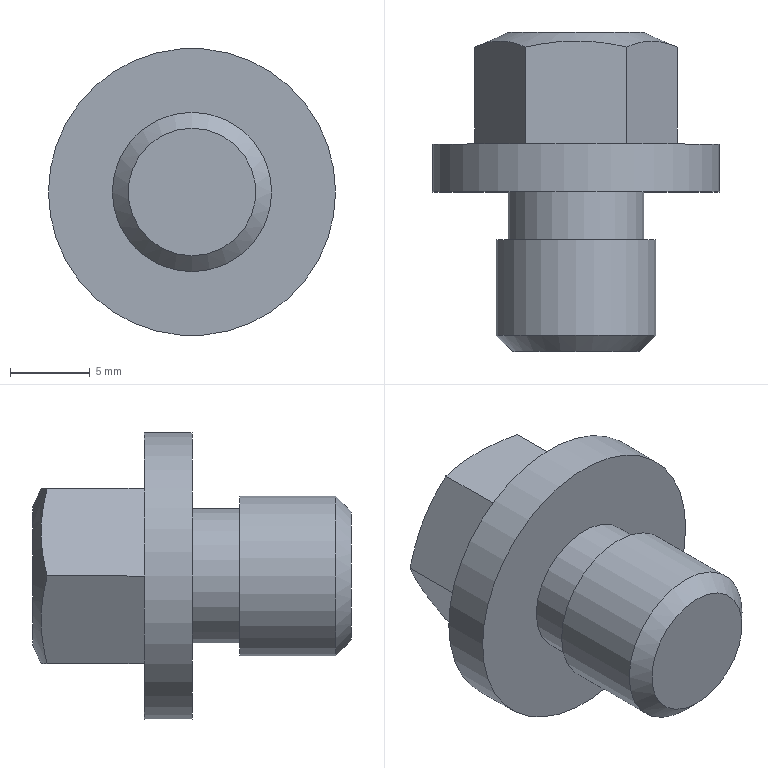Part | NX | features DATUM_CSYS 6, SKETCH 5, EXTRUDE 4, CHAMFER 1, SWP104 1 | 1 solid | 16 faces | box 18 x 20 x 18 mm | volume 2187 mm3 | plane 11 | cylinder 3 | cone 2 | commonest cylinder face diameters 8.5 x1 10 x1 18 x1
STEP:
#1=CARTESIAN_POINT('',(0.,-6.,-5.));
#2=VERTEX_POINT('',#1);
#3=CARTESIAN_POINT('',(0.,-6.,0.));
#4=DIRECTION('',(0.,-1.,0.));
#5=DIRECTION('',(0.,0.,-1.));
#6=AXIS2_PLACEMENT_3D('',#3,#4,#5);
#7=CIRCLE('',#6,5.);
#8=EDGE_CURVE('',#2,#2,#7,.F.);
#9=ORIENTED_EDGE('',*,*,#8,.T.);
#10=EDGE_LOOP('',(#9));
#11=FACE_BOUND('',#10,.T.);
#12=CARTESIAN_POINT('',(5.,0.,0.));
#13=VERTEX_POINT('',#12);
#14=CARTESIAN_POINT('',(0.,0.,0.));
#15=DIRECTION('',(0.,-1.,0.));
#16=DIRECTION('',(1.,0.,0.));
#17=AXIS2_PLACEMENT_3D('',#14,#15,#16);
#18=CIRCLE('',#17,5.);
#19=EDGE_CURVE('',#13,#13,#18,.T.);
#20=ORIENTED_EDGE('',*,*,#19,.T.);
#21=EDGE_LOOP('',(#20));
#22=FACE_BOUND('',#21,.T.);
#23=CARTESIAN_POINT('',(0.,-7.,0.));
#24=DIRECTION('',(0.,1.,0.));
#25=DIRECTION('',(0.,0.,1.));
#26=AXIS2_PLACEMENT_3D('',#23,#24,#25);
#27=CYLINDRICAL_SURFACE('',#26,5.);
#28=ADVANCED_FACE('',(#11,#22),#27,.T.);
#29=CARTESIAN_POINT('',(0.,-7.,-4.));
#30=VERTEX_POINT('',#29);
#31=CARTESIAN_POINT('',(0.,-7.,0.));
#32=DIRECTION('',(0.,-1.,0.));
#33=DIRECTION('',(0.,0.,-1.));
#34=AXIS2_PLACEMENT_3D('',#31,#32,#33);
#35=CIRCLE('',#34,4.);
#36=EDGE_CURVE('',#30,#30,#35,.T.);
#37=ORIENTED_EDGE('',*,*,#36,.T.);
#38=EDGE_LOOP('',(#37));
#39=FACE_BOUND('',#38,.T.);
#40=CARTESIAN_POINT('',(0.,-7.,0.));
#41=DIRECTION('',(0.,-1.,0.));
#42=DIRECTION('',(0.,0.,-1.));
#43=AXIS2_PLACEMENT_3D('',#40,#41,#42);
#44=PLANE('',#43);
#45=ADVANCED_FACE('',(#39),#44,.T.);
#46=CARTESIAN_POINT('',(4.25,0.,0.));
#47=VERTEX_POINT('',#46);
#48=CARTESIAN_POINT('',(0.,0.,0.));
#49=DIRECTION('',(0.,1.,0.));
#50=DIRECTION('',(1.,0.,0.));
#51=AXIS2_PLACEMENT_3D('',#48,#49,#50);
#52=CIRCLE('',#51,4.25);
#53=EDGE_CURVE('',#47,#47,#52,.T.);
#54=ORIENTED_EDGE('',*,*,#53,.F.);
#55=EDGE_LOOP('',(#54));
#56=FACE_BOUND('',#55,.T.);
#57=ORIENTED_EDGE('',*,*,#19,.F.);
#58=EDGE_LOOP('',(#57));
#59=FACE_BOUND('',#58,.T.);
#60=CARTESIAN_POINT('',(0.,0.,0.));
#61=DIRECTION('',(0.,-1.,0.));
#62=DIRECTION('',(0.,0.,-1.));
#63=AXIS2_PLACEMENT_3D('',#60,#61,#62);
#64=PLANE('',#63);
#65=ADVANCED_FACE('',(#56,#59),#64,.F.);
#66=CARTESIAN_POINT('',(4.25,3.,0.));
#67=VERTEX_POINT('',#66);
#68=CARTESIAN_POINT('',(0.,3.,0.));
#69=DIRECTION('',(0.,1.,0.));
#70=DIRECTION('',(1.,0.,0.));
#71=AXIS2_PLACEMENT_3D('',#68,#69,#70);
#72=CIRCLE('',#71,4.25);
#73=EDGE_CURVE('',#67,#67,#72,.T.);
#74=ORIENTED_EDGE('',*,*,#73,.F.);
#75=EDGE_LOOP('',(#74));
#76=FACE_BOUND('',#75,.T.);
#77=ORIENTED_EDGE('',*,*,#53,.T.);
#78=EDGE_LOOP('',(#77));
#79=FACE_BOUND('',#78,.T.);
#80=CARTESIAN_POINT('',(0.,3.,0.));
#81=DIRECTION('',(0.,-1.,0.));
#82=DIRECTION('',(0.,0.,-1.));
#83=AXIS2_PLACEMENT_3D('',#80,#81,#82);
#84=CYLINDRICAL_SURFACE('',#83,4.25);
#85=ADVANCED_FACE('',(#76,#79),#84,.T.);
#86=CARTESIAN_POINT('',(9.,6.,0.));
#87=VERTEX_POINT('',#86);
#88=CARTESIAN_POINT('',(0.,6.,0.));
#89=DIRECTION('',(0.,1.,0.));
#90=DIRECTION('',(1.,0.,0.));
#91=AXIS2_PLACEMENT_3D('',#88,#89,#90);
#92=CIRCLE('',#91,9.);
#93=EDGE_CURVE('',#87,#87,#92,.T.);
#94=ORIENTED_EDGE('',*,*,#93,.F.);
#95=EDGE_LOOP('',(#94));
#96=FACE_BOUND('',#95,.T.);
#97=CARTESIAN_POINT('',(9.,3.,0.));
#98=VERTEX_POINT('',#97);
#99=CARTESIAN_POINT('',(0.,3.,0.));
#100=DIRECTION('',(0.,1.,0.));
#101=DIRECTION('',(1.,0.,0.));
#102=AXIS2_PLACEMENT_3D('',#99,#100,#101);
#103=CIRCLE('',#102,9.);
#104=EDGE_CURVE('',#98,#98,#103,.T.);
#105=ORIENTED_EDGE('',*,*,#104,.T.);
#106=EDGE_LOOP('',(#105));
#107=FACE_BOUND('',#106,.T.);
#108=CARTESIAN_POINT('',(0.,6.,0.));
#109=DIRECTION('',(0.,-1.,0.));
#110=DIRECTION('',(0.,0.,-1.));
#111=AXIS2_PLACEMENT_3D('',#108,#109,#110);
#112=CYLINDRICAL_SURFACE('',#111,9.);
#113=ADVANCED_FACE('',(#96,#107),#112,.T.);
#114=CARTESIAN_POINT('',(-3.18,6.,-5.508));
#115=VERTEX_POINT('',#114);
#116=CARTESIAN_POINT('',(-6.36,6.,0.));
#117=VERTEX_POINT('',#116);
#118=CARTESIAN_POINT('',(-3.18,6.,-5.508));
#119=DIRECTION('',(-0.5,0.,0.866));
#120=VECTOR('',#119,1000.);
#121=LINE('',#118,#120);
#122=EDGE_CURVE('',#115,#117,#121,.T.);
#123=ORIENTED_EDGE('',*,*,#122,.F.);
#124=CARTESIAN_POINT('',(3.18,6.,-5.508));
#125=VERTEX_POINT('',#124);
#126=CARTESIAN_POINT('',(3.18,6.,-5.508));
#127=DIRECTION('',(-1.,0.,0.));
#128=VECTOR('',#127,1000.);
#129=LINE('',#126,#128);
#130=EDGE_CURVE('',#125,#115,#129,.T.);
#131=ORIENTED_EDGE('',*,*,#130,.F.);
#132=CARTESIAN_POINT('',(6.36,6.,0.));
#133=VERTEX_POINT('',#132);
#134=CARTESIAN_POINT('',(6.36,6.,0.));
#135=DIRECTION('',(-0.5,0.,-0.866));
#136=VECTOR('',#135,1000.);
#137=LINE('',#134,#136);
#138=EDGE_CURVE('',#133,#125,#137,.T.);
#139=ORIENTED_EDGE('',*,*,#138,.F.);
#140=CARTESIAN_POINT('',(3.18,6.,5.508));
#141=VERTEX_POINT('',#140);
#142=CARTESIAN_POINT('',(3.18,6.,5.508));
#143=DIRECTION('',(0.5,0.,-0.866));
#144=VECTOR('',#143,1000.);
#145=LINE('',#142,#144);
#146=EDGE_CURVE('',#141,#133,#145,.T.);
#147=ORIENTED_EDGE('',*,*,#146,.F.);
#148=CARTESIAN_POINT('',(-3.18,6.,5.508));
#149=VERTEX_POINT('',#148);
#150=CARTESIAN_POINT('',(-3.18,6.,5.508));
#151=DIRECTION('',(1.,0.,0.));
#152=VECTOR('',#151,1000.);
#153=LINE('',#150,#152);
#154=EDGE_CURVE('',#149,#141,#153,.T.);
#155=ORIENTED_EDGE('',*,*,#154,.F.);
#156=CARTESIAN_POINT('',(-6.36,6.,0.));
#157=DIRECTION('',(0.5,0.,0.866));
#158=VECTOR('',#157,1000.);
#159=LINE('',#156,#158);
#160=EDGE_CURVE('',#117,#149,#159,.T.);
#161=ORIENTED_EDGE('',*,*,#160,.F.);
#162=EDGE_LOOP('',(#123,#131,#139,#147,#155,#161));
#163=FACE_BOUND('',#162,.T.);
#164=ORIENTED_EDGE('',*,*,#93,.T.);
#165=EDGE_LOOP('',(#164));
#166=FACE_BOUND('',#165,.T.);
#167=CARTESIAN_POINT('',(0.,6.,0.));
#168=DIRECTION('',(0.,1.,0.));
#169=DIRECTION('',(0.,0.,1.));
#170=AXIS2_PLACEMENT_3D('',#167,#168,#169);
#171=PLANE('',#170);
#172=ADVANCED_FACE('',(#163,#166),#171,.T.);
#173=ORIENTED_EDGE('',*,*,#73,.T.);
#174=EDGE_LOOP('',(#173));
#175=FACE_BOUND('',#174,.T.);
#176=ORIENTED_EDGE('',*,*,#104,.F.);
#177=EDGE_LOOP('',(#176));
#178=FACE_BOUND('',#177,.T.);
#179=CARTESIAN_POINT('',(0.,3.,0.));
#180=DIRECTION('',(0.,1.,0.));
#181=DIRECTION('',(0.,0.,1.));
#182=AXIS2_PLACEMENT_3D('',#179,#180,#181);
#183=PLANE('',#182);
#184=ADVANCED_FACE('',(#175,#178),#183,.F.);
#185=CARTESIAN_POINT('',(-6.36,12.082,0.));
#186=VERTEX_POINT('',#185);
#187=CARTESIAN_POINT('',(-6.36,13.,0.));
#188=DIRECTION('',(0.,-1.,0.));
#189=VECTOR('',#188,1000.);
#190=LINE('',#187,#189);
#191=EDGE_CURVE('',#186,#117,#190,.T.);
#192=ORIENTED_EDGE('',*,*,#191,.F.);
#193=CARTESIAN_POINT('',(-3.18,12.082,-5.508));
#194=VERTEX_POINT('',#193);
#195=CARTESIAN_POINT('',(-6.36,12.082,0.));
#196=CARTESIAN_POINT('',(-5.835,12.314,-0.9096));
#197=CARTESIAN_POINT('',(-4.781,12.602,-2.734));
#198=CARTESIAN_POINT('',(-3.707,12.315,-4.595));
#199=CARTESIAN_POINT('',(-3.18,12.082,-5.508));
#200=B_SPLINE_CURVE_WITH_KNOTS('',3,(#195,#196,#197,#198,#199),.UNSPECIFIED.,.F.,.F.,(4,1,4),(0.000000233,0.003183,0.006366),.UNSPECIFIED.);
#201=EDGE_CURVE('',#186,#194,#200,.T.);
#202=ORIENTED_EDGE('',*,*,#201,.T.);
#203=CARTESIAN_POINT('',(-3.18,13.,-5.508));
#204=DIRECTION('',(0.,-1.,0.));
#205=VECTOR('',#204,1000.);
#206=LINE('',#203,#205);
#207=EDGE_CURVE('',#194,#115,#206,.T.);
#208=ORIENTED_EDGE('',*,*,#207,.T.);
#209=ORIENTED_EDGE('',*,*,#122,.T.);
#210=EDGE_LOOP('',(#192,#202,#208,#209));
#211=FACE_BOUND('',#210,.T.);
#212=CARTESIAN_POINT('',(-3.18,13.,-5.508));
#213=DIRECTION('',(0.866,0.,0.5));
#214=DIRECTION('',(0.5,0.,-0.866));
#215=AXIS2_PLACEMENT_3D('',#212,#213,#214);
#216=PLANE('',#215);
#217=ADVANCED_FACE('',(#211),#216,.F.);
#218=CARTESIAN_POINT('',(-3.18,12.082,5.508));
#219=VERTEX_POINT('',#218);
#220=CARTESIAN_POINT('',(-3.18,13.,5.508));
#221=DIRECTION('',(0.,-1.,0.));
#222=VECTOR('',#221,1000.);
#223=LINE('',#220,#222);
#224=EDGE_CURVE('',#219,#149,#223,.T.);
#225=ORIENTED_EDGE('',*,*,#224,.F.);
#226=CARTESIAN_POINT('',(-3.18,12.082,5.508));
#227=CARTESIAN_POINT('',(-3.705,12.314,4.598));
#228=CARTESIAN_POINT('',(-4.759,12.602,2.774));
#229=CARTESIAN_POINT('',(-5.833,12.315,0.9126));
#230=CARTESIAN_POINT('',(-6.36,12.082,0.));
#231=B_SPLINE_CURVE_WITH_KNOTS('',3,(#226,#227,#228,#229,#230),.UNSPECIFIED.,.F.,.F.,(4,1,4),(0.000000233,0.003183,0.006366),.UNSPECIFIED.);
#232=EDGE_CURVE('',#219,#186,#231,.T.);
#233=ORIENTED_EDGE('',*,*,#232,.T.);
#234=ORIENTED_EDGE('',*,*,#191,.T.);
#235=ORIENTED_EDGE('',*,*,#160,.T.);
#236=EDGE_LOOP('',(#225,#233,#234,#235));
#237=FACE_BOUND('',#236,.T.);
#238=CARTESIAN_POINT('',(-6.36,13.,0.));
#239=DIRECTION('',(0.866,0.,-0.5));
#240=DIRECTION('',(-0.5,0.,-0.866));
#241=AXIS2_PLACEMENT_3D('',#238,#239,#240);
#242=PLANE('',#241);
#243=ADVANCED_FACE('',(#237),#242,.F.);
#244=CARTESIAN_POINT('',(3.18,12.082,5.508));
#245=VERTEX_POINT('',#244);
#246=CARTESIAN_POINT('',(3.18,13.,5.508));
#247=DIRECTION('',(0.,-1.,0.));
#248=VECTOR('',#247,1000.);
#249=LINE('',#246,#248);
#250=EDGE_CURVE('',#245,#141,#249,.T.);
#251=ORIENTED_EDGE('',*,*,#250,.F.);
#252=CARTESIAN_POINT('',(-3.18,12.082,5.508));
#253=CARTESIAN_POINT('',(-2.133,12.313,5.508));
#254=CARTESIAN_POINT('',(-0.001857,12.604,5.508));
#255=CARTESIAN_POINT('',(2.136,12.313,5.508));
#256=CARTESIAN_POINT('',(3.18,12.082,5.508));
#257=B_SPLINE_CURVE_WITH_KNOTS('',3,(#252,#253,#254,#255,#256),.UNSPECIFIED.,.F.,.F.,(4,1,4),(0.005432,0.008641,0.01185),.UNSPECIFIED.);
#258=EDGE_CURVE('',#245,#219,#257,.F.);
#259=ORIENTED_EDGE('',*,*,#258,.T.);
#260=ORIENTED_EDGE('',*,*,#224,.T.);
#261=ORIENTED_EDGE('',*,*,#154,.T.);
#262=EDGE_LOOP('',(#251,#259,#260,#261));
#263=FACE_BOUND('',#262,.T.);
#264=CARTESIAN_POINT('',(-3.18,13.,5.508));
#265=DIRECTION('',(0.,0.,-1.));
#266=DIRECTION('',(-1.,0.,0.));
#267=AXIS2_PLACEMENT_3D('',#264,#265,#266);
#268=PLANE('',#267);
#269=ADVANCED_FACE('',(#263),#268,.F.);
#270=CARTESIAN_POINT('',(6.36,12.082,0.));
#271=VERTEX_POINT('',#270);
#272=CARTESIAN_POINT('',(6.36,13.,0.));
#273=DIRECTION('',(0.,-1.,0.));
#274=VECTOR('',#273,1000.);
#275=LINE('',#272,#274);
#276=EDGE_CURVE('',#271,#133,#275,.T.);
#277=ORIENTED_EDGE('',*,*,#276,.F.);
#278=CARTESIAN_POINT('',(6.36,12.082,0.));
#279=CARTESIAN_POINT('',(5.835,12.314,0.9096));
#280=CARTESIAN_POINT('',(4.781,12.602,2.734));
#281=CARTESIAN_POINT('',(3.707,12.315,4.595));
#282=CARTESIAN_POINT('',(3.18,12.082,5.508));
#283=B_SPLINE_CURVE_WITH_KNOTS('',3,(#278,#279,#280,#281,#282),.UNSPECIFIED.,.F.,.F.,(4,1,4),(0.000000233,0.003183,0.006366),.UNSPECIFIED.);
#284=EDGE_CURVE('',#271,#245,#283,.T.);
#285=ORIENTED_EDGE('',*,*,#284,.T.);
#286=ORIENTED_EDGE('',*,*,#250,.T.);
#287=ORIENTED_EDGE('',*,*,#146,.T.);
#288=EDGE_LOOP('',(#277,#285,#286,#287));
#289=FACE_BOUND('',#288,.T.);
#290=CARTESIAN_POINT('',(3.18,13.,5.508));
#291=DIRECTION('',(-0.866,0.,-0.5));
#292=DIRECTION('',(-0.5,0.,0.866));
#293=AXIS2_PLACEMENT_3D('',#290,#291,#292);
#294=PLANE('',#293);
#295=ADVANCED_FACE('',(#289),#294,.F.);
#296=CARTESIAN_POINT('',(3.18,12.082,-5.508));
#297=VERTEX_POINT('',#296);
#298=CARTESIAN_POINT('',(3.18,13.,-5.508));
#299=DIRECTION('',(0.,-1.,0.));
#300=VECTOR('',#299,1000.);
#301=LINE('',#298,#300);
#302=EDGE_CURVE('',#297,#125,#301,.T.);
#303=ORIENTED_EDGE('',*,*,#302,.F.);
#304=CARTESIAN_POINT('',(3.18,12.082,-5.508));
#305=CARTESIAN_POINT('',(3.705,12.314,-4.598));
#306=CARTESIAN_POINT('',(4.759,12.602,-2.774));
#307=CARTESIAN_POINT('',(5.833,12.315,-0.9126));
#308=CARTESIAN_POINT('',(6.36,12.082,0.));
#309=B_SPLINE_CURVE_WITH_KNOTS('',3,(#304,#305,#306,#307,#308),.UNSPECIFIED.,.F.,.F.,(4,1,4),(0.000000233,0.003183,0.006366),.UNSPECIFIED.);
#310=EDGE_CURVE('',#297,#271,#309,.T.);
#311=ORIENTED_EDGE('',*,*,#310,.T.);
#312=ORIENTED_EDGE('',*,*,#276,.T.);
#313=ORIENTED_EDGE('',*,*,#138,.T.);
#314=EDGE_LOOP('',(#303,#311,#312,#313));
#315=FACE_BOUND('',#314,.T.);
#316=CARTESIAN_POINT('',(6.36,13.,0.));
#317=DIRECTION('',(-0.866,0.,0.5));
#318=DIRECTION('',(0.5,0.,0.866));
#319=AXIS2_PLACEMENT_3D('',#316,#317,#318);
#320=PLANE('',#319);
#321=ADVANCED_FACE('',(#315),#320,.F.);
#322=ORIENTED_EDGE('',*,*,#207,.F.);
#323=CARTESIAN_POINT('',(-3.18,12.082,-5.508));
#324=CARTESIAN_POINT('',(-2.133,12.313,-5.508));
#325=CARTESIAN_POINT('',(-0.001857,12.604,-5.508));
#326=CARTESIAN_POINT('',(2.136,12.313,-5.508));
#327=CARTESIAN_POINT('',(3.18,12.082,-5.508));
#328=B_SPLINE_CURVE_WITH_KNOTS('',3,(#323,#324,#325,#326,#327),.UNSPECIFIED.,.F.,.F.,(4,1,4),(0.005432,0.008641,0.01185),.UNSPECIFIED.);
#329=EDGE_CURVE('',#194,#297,#328,.T.);
#330=ORIENTED_EDGE('',*,*,#329,.T.);
#331=ORIENTED_EDGE('',*,*,#302,.T.);
#332=ORIENTED_EDGE('',*,*,#130,.T.);
#333=EDGE_LOOP('',(#322,#330,#331,#332));
#334=FACE_BOUND('',#333,.T.);
#335=CARTESIAN_POINT('',(3.18,13.,-5.508));
#336=DIRECTION('',(0.,0.,1.));
#337=DIRECTION('',(1.,0.,0.));
#338=AXIS2_PLACEMENT_3D('',#335,#336,#337);
#339=PLANE('',#338);
#340=ADVANCED_FACE('',(#334),#339,.F.);
#341=CARTESIAN_POINT('',(0.,13.,-4.281));
#342=VERTEX_POINT('',#341);
#343=CARTESIAN_POINT('',(0.,13.,0.));
#344=DIRECTION('',(0.,-1.,0.));
#345=DIRECTION('',(0.,0.,-1.));
#346=AXIS2_PLACEMENT_3D('',#343,#344,#345);
#347=CIRCLE('',#346,4.281);
#348=EDGE_CURVE('',#342,#342,#347,.T.);
#349=ORIENTED_EDGE('',*,*,#348,.T.);
#350=EDGE_LOOP('',(#349));
#351=FACE_BOUND('',#350,.T.);
#352=ORIENTED_EDGE('',*,*,#232,.F.);
#353=ORIENTED_EDGE('',*,*,#258,.F.);
#354=ORIENTED_EDGE('',*,*,#284,.F.);
#355=ORIENTED_EDGE('',*,*,#310,.F.);
#356=ORIENTED_EDGE('',*,*,#329,.F.);
#357=ORIENTED_EDGE('',*,*,#201,.F.);
#358=EDGE_LOOP('',(#352,#353,#354,#355,#356,#357));
#359=FACE_BOUND('',#358,.T.);
#360=CARTESIAN_POINT('',(0.,13.,0.));
#361=DIRECTION('',(0.,-1.,0.));
#362=DIRECTION('',(0.,0.,-1.));
#363=AXIS2_PLACEMENT_3D('',#360,#361,#362);
#364=CONICAL_SURFACE('',#363,4.281,1.155);
#365=ADVANCED_FACE('',(#351,#359),#364,.T.);
#366=ORIENTED_EDGE('',*,*,#348,.F.);
#367=EDGE_LOOP('',(#366));
#368=FACE_BOUND('',#367,.T.);
#369=CARTESIAN_POINT('',(0.,13.,0.));
#370=DIRECTION('',(0.,1.,0.));
#371=DIRECTION('',(0.,0.,1.));
#372=AXIS2_PLACEMENT_3D('',#369,#370,#371);
#373=PLANE('',#372);
#374=ADVANCED_FACE('',(#368),#373,.T.);
#375=ORIENTED_EDGE('',*,*,#8,.F.);
#376=EDGE_LOOP('',(#375));
#377=FACE_BOUND('',#376,.T.);
#378=ORIENTED_EDGE('',*,*,#36,.F.);
#379=EDGE_LOOP('',(#378));
#380=FACE_BOUND('',#379,.T.);
#381=CARTESIAN_POINT('',(0.,-7.,0.));
#382=DIRECTION('',(0.,1.,0.));
#383=DIRECTION('',(0.,0.,1.));
#384=AXIS2_PLACEMENT_3D('',#381,#382,#383);
#385=CONICAL_SURFACE('',#384,4.,0.7854);
#386=ADVANCED_FACE('',(#377,#380),#385,.T.);
#387=CLOSED_SHELL('',(#28,#45,#65,#85,#113,#172,#184,#217,#243,#269,#295,#321,#340,#365,#374,#386));
#388=MANIFOLD_SOLID_BREP('',#387);
#389=(LENGTH_UNIT()NAMED_UNIT(*)SI_UNIT(.MILLI.,.METRE.));
#390=UNCERTAINTY_MEASURE_WITH_UNIT(LENGTH_MEASURE(0.0508),#389,'','');
#391=(NAMED_UNIT(*)PLANE_ANGLE_UNIT()SI_UNIT($,.RADIAN.));
#392=(NAMED_UNIT(*)SI_UNIT($,.STERADIAN.)SOLID_ANGLE_UNIT());
#393=(GEOMETRIC_REPRESENTATION_CONTEXT(3)GLOBAL_UNCERTAINTY_ASSIGNED_CONTEXT((#390))GLOBAL_UNIT_ASSIGNED_CONTEXT((#389,#391,#392))REPRESENTATION_CONTEXT('',''));
#394=ADVANCED_BREP_SHAPE_REPRESENTATION('',(#388),#393);